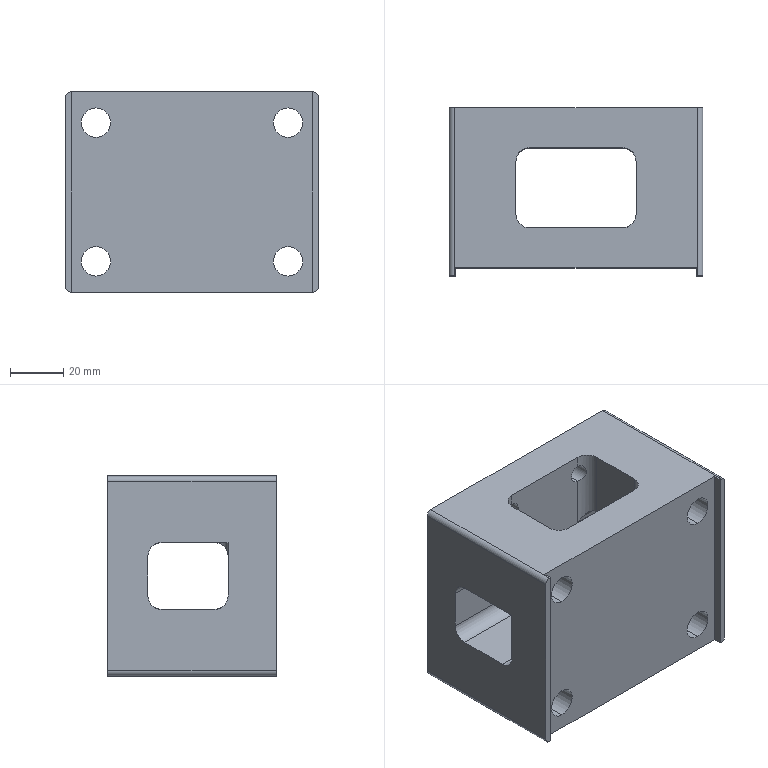Part | STEP file | 1 solid | 67 faces | box 95 x 63 x 75 mm | volume 244424 mm3 | cylinder 43 | plane 24 | commonest cylinder face diameters 10 x15 6.8 x8 11 x8 18 x8 4 x4